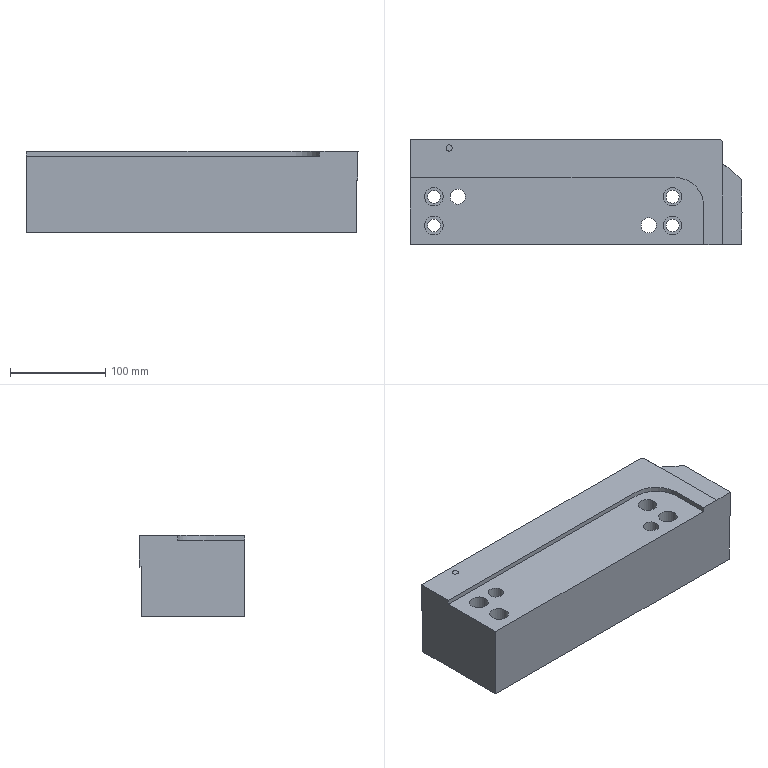Part | NX | features solid 2 | 1 solid | 27 faces | box 347.735 x 110 x 85 mm | volume 2963056 mm3 | cylinder 10 | plane 9 | spline 8 | commonest cylinder face diameters 13.5 x4 19.5 x4 16 x2